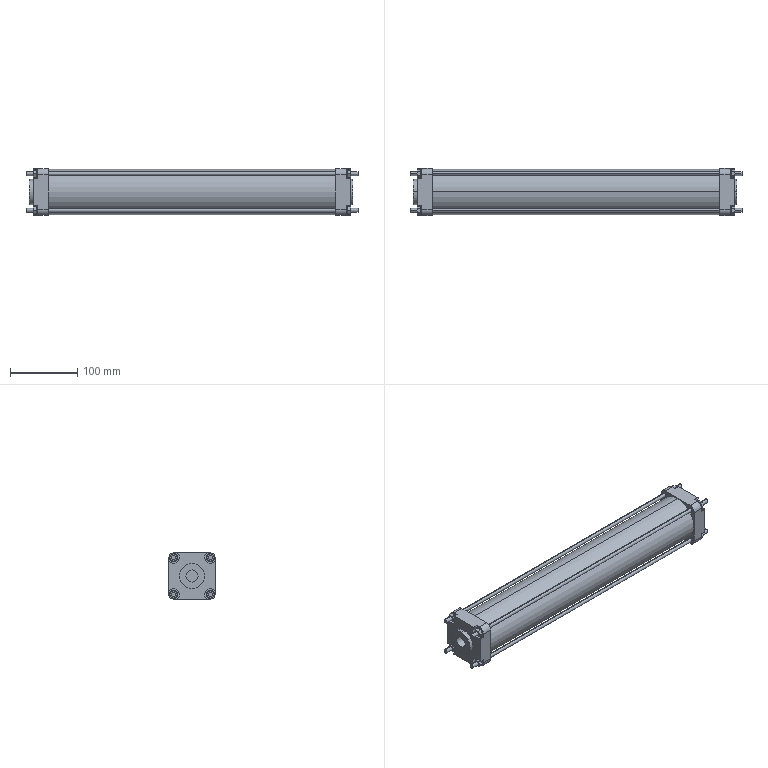Part | STEP file | _JMDBB63-400(0)_BODY | 1 solid | 206 faces | box 495 x 70 x 70 mm | volume 538960 mm3 | cylinder 102 | plane 96 | cone 8 | commonest cylinder face diameters 2 x24 6 x16 12.2 x16 17 x16 18 x10 5.3 x8